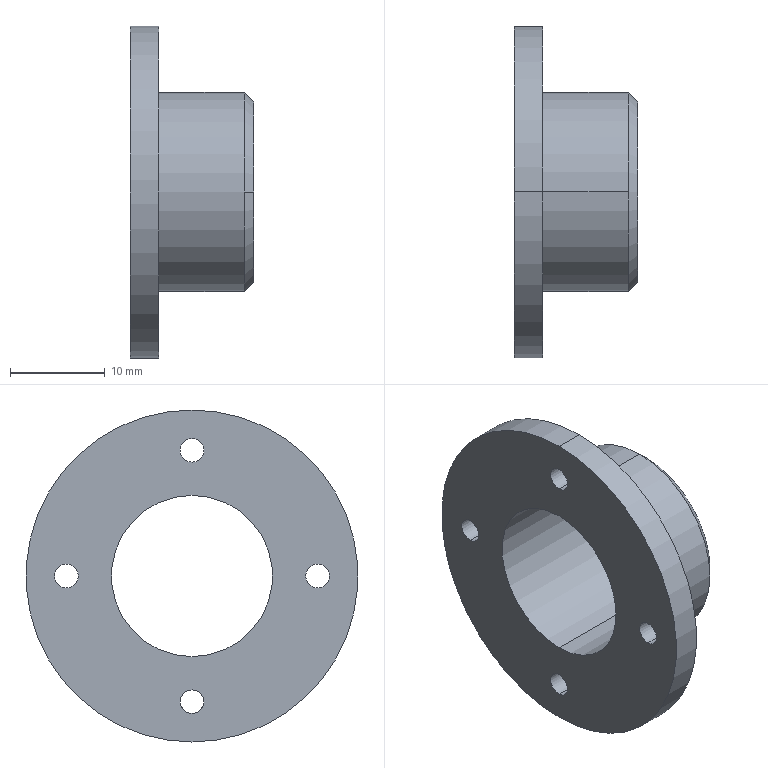Part | SolidWorks | features BaseBody 1 | 1 solid | 27 faces | box 13 x 35 x 35 mm | volume 3307 mm3 | cylinder 14 | cone 10 | plane 3 | commonest cylinder face diameters 2.5 x8 17 x2 21 x2 35 x2
STEP:
#1=CARTESIAN_POINT('',(13.,0.,-8.5));
#2=VERTEX_POINT('',#1);
#3=CARTESIAN_POINT('',(13.,0.,8.5));
#4=VERTEX_POINT('',#3);
#5=CARTESIAN_POINT('',(13.,0.,0.));
#6=DIRECTION('',(-1.,0.,0.));
#7=DIRECTION('',(0.,0.,1.));
#8=AXIS2_PLACEMENT_3D('',#5,#6,#7);
#9=CIRCLE('',#8,8.5);
#10=EDGE_CURVE('',#2,#4,#9,.T.);
#11=ORIENTED_EDGE('',*,*,#10,.F.);
#12=CARTESIAN_POINT('',(0.,0.,-8.5));
#13=VERTEX_POINT('',#12);
#14=CARTESIAN_POINT('',(3.,0.,-8.5));
#15=DIRECTION('',(-1.,0.,0.));
#16=VECTOR('',#15,1000.);
#17=LINE('',#14,#16);
#18=EDGE_CURVE('',#2,#13,#17,.T.);
#19=ORIENTED_EDGE('',*,*,#18,.T.);
#20=CARTESIAN_POINT('',(0.,0.,8.5));
#21=VERTEX_POINT('',#20);
#22=CARTESIAN_POINT('',(0.,0.,0.));
#23=DIRECTION('',(-1.,0.,0.));
#24=DIRECTION('',(0.,0.,1.));
#25=AXIS2_PLACEMENT_3D('',#22,#23,#24);
#26=CIRCLE('',#25,8.5);
#27=EDGE_CURVE('',#13,#21,#26,.T.);
#28=ORIENTED_EDGE('',*,*,#27,.T.);
#29=CARTESIAN_POINT('',(3.,0.,8.5));
#30=DIRECTION('',(-1.,0.,0.));
#31=VECTOR('',#30,1000.);
#32=LINE('',#29,#31);
#33=EDGE_CURVE('',#4,#21,#32,.T.);
#34=ORIENTED_EDGE('',*,*,#33,.F.);
#35=EDGE_LOOP('',(#11,#19,#28,#34));
#36=FACE_OUTER_BOUND('',#35,.T.);
#37=CARTESIAN_POINT('',(3.,0.,0.));
#38=DIRECTION('',(-1.,0.,0.));
#39=DIRECTION('',(0.,0.,1.));
#40=AXIS2_PLACEMENT_3D('',#37,#38,#39);
#41=CYLINDRICAL_SURFACE('',#40,8.5);
#42=ADVANCED_FACE('',(#36),#41,.F.);
#43=CARTESIAN_POINT('',(3.,0.,17.5));
#44=VERTEX_POINT('',#43);
#45=CARTESIAN_POINT('',(3.,0.,-17.5));
#46=VERTEX_POINT('',#45);
#47=CARTESIAN_POINT('',(3.,0.,0.));
#48=DIRECTION('',(-1.,0.,0.));
#49=DIRECTION('',(0.,0.,1.));
#50=AXIS2_PLACEMENT_3D('',#47,#48,#49);
#51=CIRCLE('',#50,17.5);
#52=EDGE_CURVE('',#44,#46,#51,.T.);
#53=ORIENTED_EDGE('',*,*,#52,.T.);
#54=CARTESIAN_POINT('',(0.,0.,-17.5));
#55=VERTEX_POINT('',#54);
#56=CARTESIAN_POINT('',(3.,0.,-17.5));
#57=DIRECTION('',(-1.,0.,0.));
#58=VECTOR('',#57,1000.);
#59=LINE('',#56,#58);
#60=EDGE_CURVE('',#46,#55,#59,.T.);
#61=ORIENTED_EDGE('',*,*,#60,.T.);
#62=CARTESIAN_POINT('',(0.,0.,17.5));
#63=VERTEX_POINT('',#62);
#64=CARTESIAN_POINT('',(0.,0.,0.));
#65=DIRECTION('',(1.,0.,0.));
#66=DIRECTION('',(0.,0.,1.));
#67=AXIS2_PLACEMENT_3D('',#64,#65,#66);
#68=CIRCLE('',#67,17.5);
#69=EDGE_CURVE('',#55,#63,#68,.T.);
#70=ORIENTED_EDGE('',*,*,#69,.T.);
#71=CARTESIAN_POINT('',(3.,0.,17.5));
#72=DIRECTION('',(-1.,0.,0.));
#73=VECTOR('',#72,1000.);
#74=LINE('',#71,#73);
#75=EDGE_CURVE('',#44,#63,#74,.T.);
#76=ORIENTED_EDGE('',*,*,#75,.F.);
#77=EDGE_LOOP('',(#53,#61,#70,#76));
#78=FACE_OUTER_BOUND('',#77,.T.);
#79=CARTESIAN_POINT('',(3.,0.,0.));
#80=DIRECTION('',(-1.,0.,0.));
#81=DIRECTION('',(0.,0.,1.));
#82=AXIS2_PLACEMENT_3D('',#79,#80,#81);
#83=CYLINDRICAL_SURFACE('',#82,17.5);
#84=ADVANCED_FACE('',(#78),#83,.T.);
#85=CARTESIAN_POINT('',(0.,-13.25,-1.25));
#86=VERTEX_POINT('',#85);
#87=CARTESIAN_POINT('',(0.,-13.25,1.25));
#88=VERTEX_POINT('',#87);
#89=CARTESIAN_POINT('',(0.,-13.25,0.));
#90=DIRECTION('',(-1.,0.,0.));
#91=DIRECTION('',(0.,0.,-1.));
#92=AXIS2_PLACEMENT_3D('',#89,#90,#91);
#93=CIRCLE('',#92,1.25);
#94=EDGE_CURVE('',#86,#88,#93,.T.);
#95=ORIENTED_EDGE('',*,*,#94,.T.);
#96=CARTESIAN_POINT('',(2.725,-13.25,1.25));
#97=VERTEX_POINT('',#96);
#98=CARTESIAN_POINT('',(3.,-13.25,1.25));
#99=DIRECTION('',(1.,0.,0.));
#100=VECTOR('',#99,1000.);
#101=LINE('',#98,#100);
#102=EDGE_CURVE('',#88,#97,#101,.T.);
#103=ORIENTED_EDGE('',*,*,#102,.T.);
#104=CARTESIAN_POINT('',(2.725,-13.25,-1.25));
#105=VERTEX_POINT('',#104);
#106=CARTESIAN_POINT('',(2.725,-13.25,0.));
#107=DIRECTION('',(-1.,0.,0.));
#108=DIRECTION('',(0.,0.,-1.));
#109=AXIS2_PLACEMENT_3D('',#106,#107,#108);
#110=CIRCLE('',#109,1.25);
#111=EDGE_CURVE('',#105,#97,#110,.T.);
#112=ORIENTED_EDGE('',*,*,#111,.F.);
#113=CARTESIAN_POINT('',(3.,-13.25,-1.25));
#114=DIRECTION('',(1.,0.,0.));
#115=VECTOR('',#114,1000.);
#116=LINE('',#113,#115);
#117=EDGE_CURVE('',#86,#105,#116,.T.);
#118=ORIENTED_EDGE('',*,*,#117,.F.);
#119=EDGE_LOOP('',(#95,#103,#112,#118));
#120=FACE_OUTER_BOUND('',#119,.T.);
#121=CARTESIAN_POINT('',(3.,-13.25,0.));
#122=DIRECTION('',(1.,0.,0.));
#123=DIRECTION('',(0.,0.,-1.));
#124=AXIS2_PLACEMENT_3D('',#121,#122,#123);
#125=CYLINDRICAL_SURFACE('',#124,1.25);
#126=ADVANCED_FACE('',(#120),#125,.F.);
#127=CARTESIAN_POINT('',(0.,0.,12.));
#128=VERTEX_POINT('',#127);
#129=CARTESIAN_POINT('',(0.,0.,14.5));
#130=VERTEX_POINT('',#129);
#131=CARTESIAN_POINT('',(0.,0.,13.25));
#132=DIRECTION('',(-1.,0.,0.));
#133=DIRECTION('',(0.,0.,-1.));
#134=AXIS2_PLACEMENT_3D('',#131,#132,#133);
#135=CIRCLE('',#134,1.25);
#136=EDGE_CURVE('',#128,#130,#135,.T.);
#137=ORIENTED_EDGE('',*,*,#136,.T.);
#138=CARTESIAN_POINT('',(2.725,0.,14.5));
#139=VERTEX_POINT('',#138);
#140=CARTESIAN_POINT('',(3.,0.,14.5));
#141=DIRECTION('',(1.,0.,0.));
#142=VECTOR('',#141,1000.);
#143=LINE('',#140,#142);
#144=EDGE_CURVE('',#130,#139,#143,.T.);
#145=ORIENTED_EDGE('',*,*,#144,.T.);
#146=CARTESIAN_POINT('',(2.725,0.,12.));
#147=VERTEX_POINT('',#146);
#148=CARTESIAN_POINT('',(2.725,0.,13.25));
#149=DIRECTION('',(-1.,0.,0.));
#150=DIRECTION('',(0.,0.,-1.));
#151=AXIS2_PLACEMENT_3D('',#148,#149,#150);
#152=CIRCLE('',#151,1.25);
#153=EDGE_CURVE('',#147,#139,#152,.T.);
#154=ORIENTED_EDGE('',*,*,#153,.F.);
#155=CARTESIAN_POINT('',(3.,0.,12.));
#156=DIRECTION('',(1.,0.,0.));
#157=VECTOR('',#156,1000.);
#158=LINE('',#155,#157);
#159=EDGE_CURVE('',#128,#147,#158,.T.);
#160=ORIENTED_EDGE('',*,*,#159,.F.);
#161=EDGE_LOOP('',(#137,#145,#154,#160));
#162=FACE_OUTER_BOUND('',#161,.T.);
#163=CARTESIAN_POINT('',(3.,0.,13.25));
#164=DIRECTION('',(1.,0.,0.));
#165=DIRECTION('',(0.,0.,-1.));
#166=AXIS2_PLACEMENT_3D('',#163,#164,#165);
#167=CYLINDRICAL_SURFACE('',#166,1.25);
#168=ADVANCED_FACE('',(#162),#167,.F.);
#169=CARTESIAN_POINT('',(0.,0.,-14.5));
#170=VERTEX_POINT('',#169);
#171=CARTESIAN_POINT('',(0.,0.,-12.));
#172=VERTEX_POINT('',#171);
#173=CARTESIAN_POINT('',(0.,0.,-13.25));
#174=DIRECTION('',(-1.,0.,0.));
#175=DIRECTION('',(0.,0.,-1.));
#176=AXIS2_PLACEMENT_3D('',#173,#174,#175);
#177=CIRCLE('',#176,1.25);
#178=EDGE_CURVE('',#170,#172,#177,.T.);
#179=ORIENTED_EDGE('',*,*,#178,.T.);
#180=CARTESIAN_POINT('',(2.725,0.,-12.));
#181=VERTEX_POINT('',#180);
#182=CARTESIAN_POINT('',(3.,0.,-12.));
#183=DIRECTION('',(1.,0.,0.));
#184=VECTOR('',#183,1000.);
#185=LINE('',#182,#184);
#186=EDGE_CURVE('',#172,#181,#185,.T.);
#187=ORIENTED_EDGE('',*,*,#186,.T.);
#188=CARTESIAN_POINT('',(2.725,-1.25,-13.25));
#189=VERTEX_POINT('',#188);
#190=CARTESIAN_POINT('',(2.725,0.,-13.25));
#191=DIRECTION('',(-1.,0.,0.));
#192=DIRECTION('',(0.,0.,-1.));
#193=AXIS2_PLACEMENT_3D('',#190,#191,#192);
#194=CIRCLE('',#193,1.25);
#195=EDGE_CURVE('',#189,#181,#194,.T.);
#196=ORIENTED_EDGE('',*,*,#195,.F.);
#197=CARTESIAN_POINT('',(2.725,0.,-14.5));
#198=VERTEX_POINT('',#197);
#199=CARTESIAN_POINT('',(2.725,0.,-13.25));
#200=DIRECTION('',(-1.,0.,0.));
#201=DIRECTION('',(0.,0.,-1.));
#202=AXIS2_PLACEMENT_3D('',#199,#200,#201);
#203=CIRCLE('',#202,1.25);
#204=EDGE_CURVE('',#198,#189,#203,.T.);
#205=ORIENTED_EDGE('',*,*,#204,.F.);
#206=CARTESIAN_POINT('',(3.,0.,-14.5));
#207=DIRECTION('',(1.,0.,0.));
#208=VECTOR('',#207,1000.);
#209=LINE('',#206,#208);
#210=EDGE_CURVE('',#170,#198,#209,.T.);
#211=ORIENTED_EDGE('',*,*,#210,.F.);
#212=EDGE_LOOP('',(#179,#187,#196,#205,#211));
#213=FACE_OUTER_BOUND('',#212,.T.);
#214=CARTESIAN_POINT('',(3.,0.,-13.25));
#215=DIRECTION('',(1.,0.,0.));
#216=DIRECTION('',(0.,0.,-1.));
#217=AXIS2_PLACEMENT_3D('',#214,#215,#216);
#218=CYLINDRICAL_SURFACE('',#217,1.25);
#219=ADVANCED_FACE('',(#213),#218,.F.);
#220=CARTESIAN_POINT('',(0.,13.25,-1.25));
#221=VERTEX_POINT('',#220);
#222=CARTESIAN_POINT('',(0.,13.25,1.25));
#223=VERTEX_POINT('',#222);
#224=CARTESIAN_POINT('',(0.,13.25,0.));
#225=DIRECTION('',(-1.,0.,0.));
#226=DIRECTION('',(0.,0.,-1.));
#227=AXIS2_PLACEMENT_3D('',#224,#225,#226);
#228=CIRCLE('',#227,1.25);
#229=EDGE_CURVE('',#221,#223,#228,.T.);
#230=ORIENTED_EDGE('',*,*,#229,.T.);
#231=CARTESIAN_POINT('',(2.725,13.25,1.25));
#232=VERTEX_POINT('',#231);
#233=CARTESIAN_POINT('',(3.,13.25,1.25));
#234=DIRECTION('',(1.,0.,0.));
#235=VECTOR('',#234,1000.);
#236=LINE('',#233,#235);
#237=EDGE_CURVE('',#223,#232,#236,.T.);
#238=ORIENTED_EDGE('',*,*,#237,.T.);
#239=CARTESIAN_POINT('',(2.725,13.25,-1.25));
#240=VERTEX_POINT('',#239);
#241=CARTESIAN_POINT('',(2.725,13.25,0.));
#242=DIRECTION('',(-1.,0.,0.));
#243=DIRECTION('',(0.,0.,-1.));
#244=AXIS2_PLACEMENT_3D('',#241,#242,#243);
#245=CIRCLE('',#244,1.25);
#246=EDGE_CURVE('',#240,#232,#245,.T.);
#247=ORIENTED_EDGE('',*,*,#246,.F.);
#248=CARTESIAN_POINT('',(3.,13.25,-1.25));
#249=DIRECTION('',(1.,0.,0.));
#250=VECTOR('',#249,1000.);
#251=LINE('',#248,#250);
#252=EDGE_CURVE('',#221,#240,#251,.T.);
#253=ORIENTED_EDGE('',*,*,#252,.F.);
#254=EDGE_LOOP('',(#230,#238,#247,#253));
#255=FACE_OUTER_BOUND('',#254,.T.);
#256=CARTESIAN_POINT('',(3.,13.25,0.));
#257=DIRECTION('',(1.,0.,0.));
#258=DIRECTION('',(0.,0.,-1.));
#259=AXIS2_PLACEMENT_3D('',#256,#257,#258);
#260=CYLINDRICAL_SURFACE('',#259,1.25);
#261=ADVANCED_FACE('',(#255),#260,.F.);
#262=ORIENTED_EDGE('',*,*,#111,.T.);
#263=CARTESIAN_POINT('',(3.,-13.25,1.525));
#264=VERTEX_POINT('',#263);
#265=CARTESIAN_POINT('',(3.,-13.25,1.525));
#266=DIRECTION('',(0.7071,0.,0.7071));
#267=VECTOR('',#266,1000.);
#268=LINE('',#265,#267);
#269=EDGE_CURVE('',#97,#264,#268,.T.);
#270=ORIENTED_EDGE('',*,*,#269,.T.);
#271=CARTESIAN_POINT('',(3.,-13.25,-1.525));
#272=VERTEX_POINT('',#271);
#273=CARTESIAN_POINT('',(3.,-13.25,0.));
#274=DIRECTION('',(-1.,0.,0.));
#275=DIRECTION('',(0.,0.,-1.));
#276=AXIS2_PLACEMENT_3D('',#273,#274,#275);
#277=CIRCLE('',#276,1.525);
#278=EDGE_CURVE('',#272,#264,#277,.T.);
#279=ORIENTED_EDGE('',*,*,#278,.F.);
#280=CARTESIAN_POINT('',(3.,-13.25,-1.525));
#281=DIRECTION('',(0.7071,0.,-0.7071));
#282=VECTOR('',#281,1000.);
#283=LINE('',#280,#282);
#284=EDGE_CURVE('',#105,#272,#283,.T.);
#285=ORIENTED_EDGE('',*,*,#284,.F.);
#286=EDGE_LOOP('',(#262,#270,#279,#285));
#287=FACE_OUTER_BOUND('',#286,.T.);
#288=CARTESIAN_POINT('',(3.,-13.25,0.));
#289=DIRECTION('',(1.,0.,0.));
#290=DIRECTION('',(0.,0.,-1.));
#291=AXIS2_PLACEMENT_3D('',#288,#289,#290);
#292=CONICAL_SURFACE('',#291,1.525,0.7854);
#293=ADVANCED_FACE('',(#287),#292,.F.);
#294=ORIENTED_EDGE('',*,*,#153,.T.);
#295=CARTESIAN_POINT('',(3.,0.,14.775));
#296=VERTEX_POINT('',#295);
#297=CARTESIAN_POINT('',(3.,0.,14.775));
#298=DIRECTION('',(0.7071,0.,0.7071));
#299=VECTOR('',#298,1000.);
#300=LINE('',#297,#299);
#301=EDGE_CURVE('',#139,#296,#300,.T.);
#302=ORIENTED_EDGE('',*,*,#301,.T.);
#303=CARTESIAN_POINT('',(3.,0.,11.725));
#304=VERTEX_POINT('',#303);
#305=CARTESIAN_POINT('',(3.,0.,13.25));
#306=DIRECTION('',(-1.,0.,0.));
#307=DIRECTION('',(0.,0.,-1.));
#308=AXIS2_PLACEMENT_3D('',#305,#306,#307);
#309=CIRCLE('',#308,1.525);
#310=EDGE_CURVE('',#304,#296,#309,.T.);
#311=ORIENTED_EDGE('',*,*,#310,.F.);
#312=CARTESIAN_POINT('',(3.,0.,11.725));
#313=DIRECTION('',(0.7071,0.,-0.7071));
#314=VECTOR('',#313,1000.);
#315=LINE('',#312,#314);
#316=EDGE_CURVE('',#147,#304,#315,.T.);
#317=ORIENTED_EDGE('',*,*,#316,.F.);
#318=EDGE_LOOP('',(#294,#302,#311,#317));
#319=FACE_OUTER_BOUND('',#318,.T.);
#320=CARTESIAN_POINT('',(3.,0.,13.25));
#321=DIRECTION('',(1.,0.,0.));
#322=DIRECTION('',(0.,0.,-1.));
#323=AXIS2_PLACEMENT_3D('',#320,#321,#322);
#324=CONICAL_SURFACE('',#323,1.525,0.7854);
#325=ADVANCED_FACE('',(#319),#324,.F.);
#326=CARTESIAN_POINT('',(2.725,1.25,-13.25));
#327=VERTEX_POINT('',#326);
#328=CARTESIAN_POINT('',(2.725,0.,-13.25));
#329=DIRECTION('',(-1.,0.,0.));
#330=DIRECTION('',(0.,0.,-1.));
#331=AXIS2_PLACEMENT_3D('',#328,#329,#330);
#332=CIRCLE('',#331,1.25);
#333=EDGE_CURVE('',#327,#198,#332,.T.);
#334=ORIENTED_EDGE('',*,*,#333,.T.);
#335=ORIENTED_EDGE('',*,*,#204,.T.);
#336=CARTESIAN_POINT('',(3.,-1.525,-13.25));
#337=VERTEX_POINT('',#336);
#338=CARTESIAN_POINT('',(3.,-1.525,-13.25));
#339=DIRECTION('',(0.7071,-0.7071,0.));
#340=VECTOR('',#339,1000.);
#341=LINE('',#338,#340);
#342=EDGE_CURVE('',#189,#337,#341,.T.);
#343=ORIENTED_EDGE('',*,*,#342,.T.);
#344=CARTESIAN_POINT('',(3.,1.525,-13.25));
#345=VERTEX_POINT('',#344);
#346=CARTESIAN_POINT('',(3.,0.,-13.25));
#347=DIRECTION('',(-1.,0.,0.));
#348=DIRECTION('',(0.,1.,0.));
#349=AXIS2_PLACEMENT_3D('',#346,#347,#348);
#350=CIRCLE('',#349,1.525);
#351=EDGE_CURVE('',#345,#337,#350,.T.);
#352=ORIENTED_EDGE('',*,*,#351,.F.);
#353=CARTESIAN_POINT('',(3.,1.525,-13.25));
#354=DIRECTION('',(0.7071,0.7071,0.));
#355=VECTOR('',#354,1000.);
#356=LINE('',#353,#355);
#357=EDGE_CURVE('',#327,#345,#356,.T.);
#358=ORIENTED_EDGE('',*,*,#357,.F.);
#359=EDGE_LOOP('',(#334,#335,#343,#352,#358));
#360=FACE_OUTER_BOUND('',#359,.T.);
#361=CARTESIAN_POINT('',(3.,0.,-13.25));
#362=DIRECTION('',(1.,0.,0.));
#363=DIRECTION('',(0.,1.,0.));
#364=AXIS2_PLACEMENT_3D('',#361,#362,#363);
#365=CONICAL_SURFACE('',#364,1.525,0.7854);
#366=ADVANCED_FACE('',(#360),#365,.F.);
#367=ORIENTED_EDGE('',*,*,#246,.T.);
#368=CARTESIAN_POINT('',(3.,13.25,1.525));
#369=VERTEX_POINT('',#368);
#370=CARTESIAN_POINT('',(3.,13.25,1.525));
#371=DIRECTION('',(0.7071,0.,0.7071));
#372=VECTOR('',#371,1000.);
#373=LINE('',#370,#372);
#374=EDGE_CURVE('',#232,#369,#373,.T.);
#375=ORIENTED_EDGE('',*,*,#374,.T.);
#376=CARTESIAN_POINT('',(3.,13.25,-1.525));
#377=VERTEX_POINT('',#376);
#378=CARTESIAN_POINT('',(3.,13.25,0.));
#379=DIRECTION('',(-1.,0.,0.));
#380=DIRECTION('',(0.,0.,-1.));
#381=AXIS2_PLACEMENT_3D('',#378,#379,#380);
#382=CIRCLE('',#381,1.525);
#383=EDGE_CURVE('',#377,#369,#382,.T.);
#384=ORIENTED_EDGE('',*,*,#383,.F.);
#385=CARTESIAN_POINT('',(3.,13.25,-1.525));
#386=DIRECTION('',(0.7071,0.,-0.7071));
#387=VECTOR('',#386,1000.);
#388=LINE('',#385,#387);
#389=EDGE_CURVE('',#240,#377,#388,.T.);
#390=ORIENTED_EDGE('',*,*,#389,.F.);
#391=EDGE_LOOP('',(#367,#375,#384,#390));
#392=FACE_OUTER_BOUND('',#391,.T.);
#393=CARTESIAN_POINT('',(3.,13.25,0.));
#394=DIRECTION('',(1.,0.,0.));
#395=DIRECTION('',(0.,0.,-1.));
#396=AXIS2_PLACEMENT_3D('',#393,#394,#395);
#397=CONICAL_SURFACE('',#396,1.525,0.7854);
#398=ADVANCED_FACE('',(#392),#397,.F.);
#399=CARTESIAN_POINT('',(13.,9.5,0.));
#400=VERTEX_POINT('',#399);
#401=CARTESIAN_POINT('',(13.,-9.5,0.));
#402=VERTEX_POINT('',#401);
#403=CARTESIAN_POINT('',(13.,0.,0.));
#404=DIRECTION('',(1.,0.,0.));
#405=DIRECTION('',(0.,-1.,0.));
#406=AXIS2_PLACEMENT_3D('',#403,#404,#405);
#407=CIRCLE('',#406,9.5);
#408=EDGE_CURVE('',#400,#402,#407,.T.);
#409=ORIENTED_EDGE('',*,*,#408,.F.);
#410=CARTESIAN_POINT('',(12.,10.5,0.));
#411=VERTEX_POINT('',#410);
#412=CARTESIAN_POINT('',(12.,10.5,0.));
#413=DIRECTION('',(-0.7071,0.7071,0.));
#414=VECTOR('',#413,1000.);
#415=LINE('',#412,#414);
#416=EDGE_CURVE('',#400,#411,#415,.T.);
#417=ORIENTED_EDGE('',*,*,#416,.T.);
#418=CARTESIAN_POINT('',(12.,0.,10.5));
#419=VERTEX_POINT('',#418);
#420=CARTESIAN_POINT('',(12.,0.,0.));
#421=DIRECTION('',(1.,0.,0.));
#422=DIRECTION('',(0.,0.,1.));
#423=AXIS2_PLACEMENT_3D('',#420,#421,#422);
#424=CIRCLE('',#423,10.5);
#425=EDGE_CURVE('',#411,#419,#424,.T.);
#426=ORIENTED_EDGE('',*,*,#425,.T.);
#427=CARTESIAN_POINT('',(12.,-10.5,0.));
#428=VERTEX_POINT('',#427);
#429=CARTESIAN_POINT('',(12.,0.,0.));
#430=DIRECTION('',(1.,0.,0.));
#431=DIRECTION('',(0.,0.,1.));
#432=AXIS2_PLACEMENT_3D('',#429,#430,#431);
#433=CIRCLE('',#432,10.5);
#434=EDGE_CURVE('',#419,#428,#433,.T.);
#435=ORIENTED_EDGE('',*,*,#434,.T.);
#436=CARTESIAN_POINT('',(12.,-10.5,0.));
#437=DIRECTION('',(-0.7071,-0.7071,0.));
#438=VECTOR('',#437,1000.);
#439=LINE('',#436,#438);
#440=EDGE_CURVE('',#402,#428,#439,.T.);
#441=ORIENTED_EDGE('',*,*,#440,.F.);
#442=EDGE_LOOP('',(#409,#417,#426,#435,#441));
#443=FACE_OUTER_BOUND('',#442,.T.);
#444=CARTESIAN_POINT('',(12.,0.,0.));
#445=DIRECTION('',(-1.,0.,0.));
#446=DIRECTION('',(0.,-1.,0.));
#447=AXIS2_PLACEMENT_3D('',#444,#445,#446);
#448=CONICAL_SURFACE('',#447,10.5,0.7854);
#449=ADVANCED_FACE('',(#443),#448,.T.);
#450=CARTESIAN_POINT('',(12.,0.,-10.5));
#451=VERTEX_POINT('',#450);
#452=CARTESIAN_POINT('',(12.,0.,0.));
#453=DIRECTION('',(1.,0.,0.));
#454=DIRECTION('',(0.,0.,1.));
#455=AXIS2_PLACEMENT_3D('',#452,#453,#454);
#456=CIRCLE('',#455,10.5);
#457=EDGE_CURVE('',#451,#411,#456,.T.);
#458=ORIENTED_EDGE('',*,*,#457,.F.);
#459=CARTESIAN_POINT('',(3.,0.,-10.5));
#460=VERTEX_POINT('',#459);
#461=CARTESIAN_POINT('',(13.,0.,-10.5));
#462=DIRECTION('',(-1.,0.,0.));
#463=VECTOR('',#462,1000.);
#464=LINE('',#461,#463);
#465=EDGE_CURVE('',#451,#460,#464,.T.);
#466=ORIENTED_EDGE('',*,*,#465,.T.);
#467=CARTESIAN_POINT('',(3.,0.,10.5));
#468=VERTEX_POINT('',#467);
#469=CARTESIAN_POINT('',(3.,0.,0.));
#470=DIRECTION('',(-1.,0.,0.));
#471=DIRECTION('',(0.,0.,1.));
#472=AXIS2_PLACEMENT_3D('',#469,#470,#471);
#473=CIRCLE('',#472,10.5);
#474=EDGE_CURVE('',#468,#460,#473,.T.);
#475=ORIENTED_EDGE('',*,*,#474,.F.);
#476=CARTESIAN_POINT('',(13.,0.,10.5));
#477=DIRECTION('',(-1.,0.,0.));
#478=VECTOR('',#477,1000.);
#479=LINE('',#476,#478);
#480=EDGE_CURVE('',#419,#468,#479,.T.);
#481=ORIENTED_EDGE('',*,*,#480,.F.);
#482=ORIENTED_EDGE('',*,*,#425,.F.);
#483=EDGE_LOOP('',(#458,#466,#475,#481,#482));
#484=FACE_OUTER_BOUND('',#483,.T.);
#485=CARTESIAN_POINT('',(13.,0.,0.));
#486=DIRECTION('',(-1.,0.,0.));
#487=DIRECTION('',(0.,0.,1.));
#488=AXIS2_PLACEMENT_3D('',#485,#486,#487);
#489=CYLINDRICAL_SURFACE('',#488,10.5);
#490=ADVANCED_FACE('',(#484),#489,.T.);
#491=CARTESIAN_POINT('',(0.,0.,0.));
#492=DIRECTION('',(-1.,0.,0.));
#493=DIRECTION('',(0.,0.,1.));
#494=AXIS2_PLACEMENT_3D('',#491,#492,#493);
#495=CIRCLE('',#494,8.5);
#496=EDGE_CURVE('',#21,#13,#495,.T.);
#497=ORIENTED_EDGE('',*,*,#496,.F.);
#498=ORIENTED_EDGE('',*,*,#27,.F.);
#499=EDGE_LOOP('',(#497,#498));
#500=FACE_BOUND('',#499,.T.);
#501=CARTESIAN_POINT('',(0.,0.,0.));
#502=DIRECTION('',(1.,0.,0.));
#503=DIRECTION('',(0.,0.,1.));
#504=AXIS2_PLACEMENT_3D('',#501,#502,#503);
#505=CIRCLE('',#504,17.5);
#506=EDGE_CURVE('',#63,#55,#505,.T.);
#507=ORIENTED_EDGE('',*,*,#506,.F.);
#508=ORIENTED_EDGE('',*,*,#69,.F.);
#509=EDGE_LOOP('',(#507,#508));
#510=FACE_OUTER_BOUND('',#509,.T.);
#511=ORIENTED_EDGE('',*,*,#94,.F.);
#512=CARTESIAN_POINT('',(0.,-13.25,0.));
#513=DIRECTION('',(-1.,0.,0.));
#514=DIRECTION('',(0.,0.,-1.));
#515=AXIS2_PLACEMENT_3D('',#512,#513,#514);
#516=CIRCLE('',#515,1.25);
#517=EDGE_CURVE('',#88,#86,#516,.T.);
#518=ORIENTED_EDGE('',*,*,#517,.F.);
#519=EDGE_LOOP('',(#511,#518));
#520=FACE_BOUND('',#519,.T.);
#521=ORIENTED_EDGE('',*,*,#136,.F.);
#522=CARTESIAN_POINT('',(0.,0.,13.25));
#523=DIRECTION('',(-1.,0.,0.));
#524=DIRECTION('',(0.,0.,-1.));
#525=AXIS2_PLACEMENT_3D('',#522,#523,#524);
#526=CIRCLE('',#525,1.25);
#527=EDGE_CURVE('',#130,#128,#526,.T.);
#528=ORIENTED_EDGE('',*,*,#527,.F.);
#529=EDGE_LOOP('',(#521,#528));
#530=FACE_BOUND('',#529,.T.);
#531=ORIENTED_EDGE('',*,*,#178,.F.);
#532=CARTESIAN_POINT('',(0.,0.,-13.25));
#533=DIRECTION('',(-1.,0.,0.));
#534=DIRECTION('',(0.,0.,-1.));
#535=AXIS2_PLACEMENT_3D('',#532,#533,#534);
#536=CIRCLE('',#535,1.25);
#537=EDGE_CURVE('',#172,#170,#536,.T.);
#538=ORIENTED_EDGE('',*,*,#537,.F.);
#539=EDGE_LOOP('',(#531,#538));
#540=FACE_BOUND('',#539,.T.);
#541=ORIENTED_EDGE('',*,*,#229,.F.);
#542=CARTESIAN_POINT('',(0.,13.25,0.));
#543=DIRECTION('',(-1.,0.,0.));
#544=DIRECTION('',(0.,0.,-1.));
#545=AXIS2_PLACEMENT_3D('',#542,#543,#544);
#546=CIRCLE('',#545,1.25);
#547=EDGE_CURVE('',#223,#221,#546,.T.);
#548=ORIENTED_EDGE('',*,*,#547,.F.);
#549=EDGE_LOOP('',(#541,#548));
#550=FACE_BOUND('',#549,.T.);
#551=CARTESIAN_POINT('',(0.,0.,0.));
#552=DIRECTION('',(1.,0.,0.));
#553=DIRECTION('',(0.,0.,-1.));
#554=AXIS2_PLACEMENT_3D('',#551,#552,#553);
#555=PLANE('',#554);
#556=ADVANCED_FACE('',(#500,#510,#520,#530,#540,#550),#555,.F.);
#557=ORIENTED_EDGE('',*,*,#18,.F.);
#558=CARTESIAN_POINT('',(13.,0.,0.));
#559=DIRECTION('',(-1.,0.,0.));
#560=DIRECTION('',(0.,0.,1.));
#561=AXIS2_PLACEMENT_3D('',#558,#559,#560);
#562=CIRCLE('',#561,8.5);
#563=EDGE_CURVE('',#4,#2,#562,.T.);
#564=ORIENTED_EDGE('',*,*,#563,.F.);
#565=ORIENTED_EDGE('',*,*,#33,.T.);
#566=ORIENTED_EDGE('',*,*,#496,.T.);
#567=EDGE_LOOP('',(#557,#564,#565,#566));
#568=FACE_OUTER_BOUND('',#567,.T.);
#569=CARTESIAN_POINT('',(3.,0.,0.));
#570=DIRECTION('',(-1.,0.,0.));
#571=DIRECTION('',(0.,0.,1.));
#572=AXIS2_PLACEMENT_3D('',#569,#570,#571);
#573=CYLINDRICAL_SURFACE('',#572,8.5);
#574=ADVANCED_FACE('',(#568),#573,.F.);
#575=ORIENTED_EDGE('',*,*,#60,.F.);
#576=CARTESIAN_POINT('',(3.,0.,0.));
#577=DIRECTION('',(-1.,0.,0.));
#578=DIRECTION('',(0.,0.,1.));
#579=AXIS2_PLACEMENT_3D('',#576,#577,#578);
#580=CIRCLE('',#579,17.5);
#581=EDGE_CURVE('',#46,#44,#580,.T.);
#582=ORIENTED_EDGE('',*,*,#581,.T.);
#583=ORIENTED_EDGE('',*,*,#75,.T.);
#584=ORIENTED_EDGE('',*,*,#506,.T.);
#585=EDGE_LOOP('',(#575,#582,#583,#584));
#586=FACE_OUTER_BOUND('',#585,.T.);
#587=CARTESIAN_POINT('',(3.,0.,0.));
#588=DIRECTION('',(-1.,0.,0.));
#589=DIRECTION('',(0.,0.,1.));
#590=AXIS2_PLACEMENT_3D('',#587,#588,#589);
#591=CYLINDRICAL_SURFACE('',#590,17.5);
#592=ADVANCED_FACE('',(#586),#591,.T.);
#593=ORIENTED_EDGE('',*,*,#102,.F.);
#594=ORIENTED_EDGE('',*,*,#517,.T.);
#595=ORIENTED_EDGE('',*,*,#117,.T.);
#596=CARTESIAN_POINT('',(2.725,-13.25,0.));
#597=DIRECTION('',(-1.,0.,0.));
#598=DIRECTION('',(0.,0.,-1.));
#599=AXIS2_PLACEMENT_3D('',#596,#597,#598);
#600=CIRCLE('',#599,1.25);
#601=EDGE_CURVE('',#97,#105,#600,.T.);
#602=ORIENTED_EDGE('',*,*,#601,.F.);
#603=EDGE_LOOP('',(#593,#594,#595,#602));
#604=FACE_OUTER_BOUND('',#603,.T.);
#605=CARTESIAN_POINT('',(3.,-13.25,0.));
#606=DIRECTION('',(1.,0.,0.));
#607=DIRECTION('',(0.,0.,-1.));
#608=AXIS2_PLACEMENT_3D('',#605,#606,#607);
#609=CYLINDRICAL_SURFACE('',#608,1.25);
#610=ADVANCED_FACE('',(#604),#609,.F.);
#611=ORIENTED_EDGE('',*,*,#144,.F.);
#612=ORIENTED_EDGE('',*,*,#527,.T.);
#613=ORIENTED_EDGE('',*,*,#159,.T.);
#614=CARTESIAN_POINT('',(2.725,0.,13.25));
#615=DIRECTION('',(-1.,0.,0.));
#616=DIRECTION('',(0.,0.,-1.));
#617=AXIS2_PLACEMENT_3D('',#614,#615,#616);
#618=CIRCLE('',#617,1.25);
#619=EDGE_CURVE('',#139,#147,#618,.T.);
#620=ORIENTED_EDGE('',*,*,#619,.F.);
#621=EDGE_LOOP('',(#611,#612,#613,#620));
#622=FACE_OUTER_BOUND('',#621,.T.);
#623=CARTESIAN_POINT('',(3.,0.,13.25));
#624=DIRECTION('',(1.,0.,0.));
#625=DIRECTION('',(0.,0.,-1.));
#626=AXIS2_PLACEMENT_3D('',#623,#624,#625);
#627=CYLINDRICAL_SURFACE('',#626,1.25);
#628=ADVANCED_FACE('',(#622),#627,.F.);
#629=ORIENTED_EDGE('',*,*,#186,.F.);
#630=ORIENTED_EDGE('',*,*,#537,.T.);
#631=ORIENTED_EDGE('',*,*,#210,.T.);
#632=ORIENTED_EDGE('',*,*,#333,.F.);
#633=CARTESIAN_POINT('',(2.725,0.,-13.25));
#634=DIRECTION('',(-1.,0.,0.));
#635=DIRECTION('',(0.,0.,-1.));
#636=AXIS2_PLACEMENT_3D('',#633,#634,#635);
#637=CIRCLE('',#636,1.25);
#638=EDGE_CURVE('',#181,#327,#637,.T.);
#639=ORIENTED_EDGE('',*,*,#638,.F.);
#640=EDGE_LOOP('',(#629,#630,#631,#632,#639));
#641=FACE_OUTER_BOUND('',#640,.T.);
#642=CARTESIAN_POINT('',(3.,0.,-13.25));
#643=DIRECTION('',(1.,0.,0.));
#644=DIRECTION('',(0.,0.,-1.));
#645=AXIS2_PLACEMENT_3D('',#642,#643,#644);
#646=CYLINDRICAL_SURFACE('',#645,1.25);
#647=ADVANCED_FACE('',(#641),#646,.F.);
#648=ORIENTED_EDGE('',*,*,#237,.F.);
#649=ORIENTED_EDGE('',*,*,#547,.T.);
#650=ORIENTED_EDGE('',*,*,#252,.T.);
#651=CARTESIAN_POINT('',(2.725,13.25,0.));
#652=DIRECTION('',(-1.,0.,0.));
#653=DIRECTION('',(0.,0.,-1.));
#654=AXIS2_PLACEMENT_3D('',#651,#652,#653);
#655=CIRCLE('',#654,1.25);
#656=EDGE_CURVE('',#232,#240,#655,.T.);
#657=ORIENTED_EDGE('',*,*,#656,.F.);
#658=EDGE_LOOP('',(#648,#649,#650,#657));
#659=FACE_OUTER_BOUND('',#658,.T.);
#660=CARTESIAN_POINT('',(3.,13.25,0.));
#661=DIRECTION('',(1.,0.,0.));
#662=DIRECTION('',(0.,0.,-1.));
#663=AXIS2_PLACEMENT_3D('',#660,#661,#662);
#664=CYLINDRICAL_SURFACE('',#663,1.25);
#665=ADVANCED_FACE('',(#659),#664,.F.);
#666=ORIENTED_EDGE('',*,*,#563,.T.);
#667=ORIENTED_EDGE('',*,*,#10,.T.);
#668=EDGE_LOOP('',(#666,#667));
#669=FACE_BOUND('',#668,.T.);
#670=CARTESIAN_POINT('',(13.,0.,0.));
#671=DIRECTION('',(1.,0.,0.));
#672=DIRECTION('',(0.,-1.,0.));
#673=AXIS2_PLACEMENT_3D('',#670,#671,#672);
#674=CIRCLE('',#673,9.5);
#675=EDGE_CURVE('',#402,#400,#674,.T.);
#676=ORIENTED_EDGE('',*,*,#675,.T.);
#677=ORIENTED_EDGE('',*,*,#408,.T.);
#678=EDGE_LOOP('',(#676,#677));
#679=FACE_OUTER_BOUND('',#678,.T.);
#680=CARTESIAN_POINT('',(13.,0.,0.));
#681=DIRECTION('',(1.,0.,0.));
#682=DIRECTION('',(0.,0.,-1.));
#683=AXIS2_PLACEMENT_3D('',#680,#681,#682);
#684=PLANE('',#683);
#685=ADVANCED_FACE('',(#669,#679),#684,.T.);
#686=ORIENTED_EDGE('',*,*,#474,.T.);
#687=CARTESIAN_POINT('',(3.,0.,0.));
#688=DIRECTION('',(-1.,0.,0.));
#689=DIRECTION('',(0.,0.,1.));
#690=AXIS2_PLACEMENT_3D('',#687,#688,#689);
#691=CIRCLE('',#690,10.5);
#692=EDGE_CURVE('',#460,#468,#691,.T.);
#693=ORIENTED_EDGE('',*,*,#692,.T.);
#694=EDGE_LOOP('',(#686,#693));
#695=FACE_BOUND('',#694,.T.);
#696=ORIENTED_EDGE('',*,*,#52,.F.);
#697=ORIENTED_EDGE('',*,*,#581,.F.);
#698=EDGE_LOOP('',(#696,#697));
#699=FACE_OUTER_BOUND('',#698,.T.);
#700=ORIENTED_EDGE('',*,*,#278,.T.);
#701=CARTESIAN_POINT('',(3.,-13.25,0.));
#702=DIRECTION('',(-1.,0.,0.));
#703=DIRECTION('',(0.,0.,-1.));
#704=AXIS2_PLACEMENT_3D('',#701,#702,#703);
#705=CIRCLE('',#704,1.525);
#706=EDGE_CURVE('',#264,#272,#705,.T.);
#707=ORIENTED_EDGE('',*,*,#706,.T.);
#708=EDGE_LOOP('',(#700,#707));
#709=FACE_BOUND('',#708,.T.);
#710=ORIENTED_EDGE('',*,*,#310,.T.);
#711=CARTESIAN_POINT('',(3.,0.,13.25));
#712=DIRECTION('',(-1.,0.,0.));
#713=DIRECTION('',(0.,0.,-1.));
#714=AXIS2_PLACEMENT_3D('',#711,#712,#713);
#715=CIRCLE('',#714,1.525);
#716=EDGE_CURVE('',#296,#304,#715,.T.);
#717=ORIENTED_EDGE('',*,*,#716,.T.);
#718=EDGE_LOOP('',(#710,#717));
#719=FACE_BOUND('',#718,.T.);
#720=ORIENTED_EDGE('',*,*,#351,.T.);
#721=CARTESIAN_POINT('',(3.,0.,-13.25));
#722=DIRECTION('',(-1.,0.,0.));
#723=DIRECTION('',(0.,1.,0.));
#724=AXIS2_PLACEMENT_3D('',#721,#722,#723);
#725=CIRCLE('',#724,1.525);
#726=EDGE_CURVE('',#337,#345,#725,.T.);
#727=ORIENTED_EDGE('',*,*,#726,.T.);
#728=EDGE_LOOP('',(#720,#727));
#729=FACE_BOUND('',#728,.T.);
#730=ORIENTED_EDGE('',*,*,#383,.T.);
#731=CARTESIAN_POINT('',(3.,13.25,0.));
#732=DIRECTION('',(-1.,0.,0.));
#733=DIRECTION('',(0.,0.,-1.));
#734=AXIS2_PLACEMENT_3D('',#731,#732,#733);
#735=CIRCLE('',#734,1.525);
#736=EDGE_CURVE('',#369,#377,#735,.T.);
#737=ORIENTED_EDGE('',*,*,#736,.T.);
#738=EDGE_LOOP('',(#730,#737));
#739=FACE_BOUND('',#738,.T.);
#740=CARTESIAN_POINT('',(3.,0.,0.));
#741=DIRECTION('',(1.,0.,0.));
#742=DIRECTION('',(0.,0.,-1.));
#743=AXIS2_PLACEMENT_3D('',#740,#741,#742);
#744=PLANE('',#743);
#745=ADVANCED_FACE('',(#695,#699,#709,#719,#729,#739),#744,.T.);
#746=ORIENTED_EDGE('',*,*,#269,.F.);
#747=ORIENTED_EDGE('',*,*,#601,.T.);
#748=ORIENTED_EDGE('',*,*,#284,.T.);
#749=ORIENTED_EDGE('',*,*,#706,.F.);
#750=EDGE_LOOP('',(#746,#747,#748,#749));
#751=FACE_OUTER_BOUND('',#750,.T.);
#752=CARTESIAN_POINT('',(3.,-13.25,0.));
#753=DIRECTION('',(1.,0.,0.));
#754=DIRECTION('',(0.,0.,-1.));
#755=AXIS2_PLACEMENT_3D('',#752,#753,#754);
#756=CONICAL_SURFACE('',#755,1.525,0.7854);
#757=ADVANCED_FACE('',(#751),#756,.F.);
#758=ORIENTED_EDGE('',*,*,#301,.F.);
#759=ORIENTED_EDGE('',*,*,#619,.T.);
#760=ORIENTED_EDGE('',*,*,#316,.T.);
#761=ORIENTED_EDGE('',*,*,#716,.F.);
#762=EDGE_LOOP('',(#758,#759,#760,#761));
#763=FACE_OUTER_BOUND('',#762,.T.);
#764=CARTESIAN_POINT('',(3.,0.,13.25));
#765=DIRECTION('',(1.,0.,0.));
#766=DIRECTION('',(0.,0.,-1.));
#767=AXIS2_PLACEMENT_3D('',#764,#765,#766);
#768=CONICAL_SURFACE('',#767,1.525,0.7854);
#769=ADVANCED_FACE('',(#763),#768,.F.);
#770=ORIENTED_EDGE('',*,*,#342,.F.);
#771=ORIENTED_EDGE('',*,*,#195,.T.);
#772=ORIENTED_EDGE('',*,*,#638,.T.);
#773=ORIENTED_EDGE('',*,*,#357,.T.);
#774=ORIENTED_EDGE('',*,*,#726,.F.);
#775=EDGE_LOOP('',(#770,#771,#772,#773,#774));
#776=FACE_OUTER_BOUND('',#775,.T.);
#777=CARTESIAN_POINT('',(3.,0.,-13.25));
#778=DIRECTION('',(1.,0.,0.));
#779=DIRECTION('',(0.,1.,0.));
#780=AXIS2_PLACEMENT_3D('',#777,#778,#779);
#781=CONICAL_SURFACE('',#780,1.525,0.7854);
#782=ADVANCED_FACE('',(#776),#781,.F.);
#783=ORIENTED_EDGE('',*,*,#374,.F.);
#784=ORIENTED_EDGE('',*,*,#656,.T.);
#785=ORIENTED_EDGE('',*,*,#389,.T.);
#786=ORIENTED_EDGE('',*,*,#736,.F.);
#787=EDGE_LOOP('',(#783,#784,#785,#786));
#788=FACE_OUTER_BOUND('',#787,.T.);
#789=CARTESIAN_POINT('',(3.,13.25,0.));
#790=DIRECTION('',(1.,0.,0.));
#791=DIRECTION('',(0.,0.,-1.));
#792=AXIS2_PLACEMENT_3D('',#789,#790,#791);
#793=CONICAL_SURFACE('',#792,1.525,0.7854);
#794=ADVANCED_FACE('',(#788),#793,.F.);
#795=ORIENTED_EDGE('',*,*,#416,.F.);
#796=ORIENTED_EDGE('',*,*,#675,.F.);
#797=ORIENTED_EDGE('',*,*,#440,.T.);
#798=CARTESIAN_POINT('',(12.,0.,0.));
#799=DIRECTION('',(1.,0.,0.));
#800=DIRECTION('',(0.,0.,1.));
#801=AXIS2_PLACEMENT_3D('',#798,#799,#800);
#802=CIRCLE('',#801,10.5);
#803=EDGE_CURVE('',#428,#451,#802,.T.);
#804=ORIENTED_EDGE('',*,*,#803,.T.);
#805=ORIENTED_EDGE('',*,*,#457,.T.);
#806=EDGE_LOOP('',(#795,#796,#797,#804,#805));
#807=FACE_OUTER_BOUND('',#806,.T.);
#808=CARTESIAN_POINT('',(12.,0.,0.));
#809=DIRECTION('',(-1.,0.,0.));
#810=DIRECTION('',(0.,-1.,0.));
#811=AXIS2_PLACEMENT_3D('',#808,#809,#810);
#812=CONICAL_SURFACE('',#811,10.5,0.7854);
#813=ADVANCED_FACE('',(#807),#812,.T.);
#814=ORIENTED_EDGE('',*,*,#465,.F.);
#815=ORIENTED_EDGE('',*,*,#803,.F.);
#816=ORIENTED_EDGE('',*,*,#434,.F.);
#817=ORIENTED_EDGE('',*,*,#480,.T.);
#818=ORIENTED_EDGE('',*,*,#692,.F.);
#819=EDGE_LOOP('',(#814,#815,#816,#817,#818));
#820=FACE_OUTER_BOUND('',#819,.T.);
#821=CARTESIAN_POINT('',(13.,0.,0.));
#822=DIRECTION('',(-1.,0.,0.));
#823=DIRECTION('',(0.,0.,1.));
#824=AXIS2_PLACEMENT_3D('',#821,#822,#823);
#825=CYLINDRICAL_SURFACE('',#824,10.5);
#826=ADVANCED_FACE('',(#820),#825,.T.);
#827=CLOSED_SHELL('',(#42,#84,#126,#168,#219,#261,#293,#325,#366,#398,#449,#490,#556,#574,#592,#610,#628,#647,#665,#685,#745,#757,#769,#782,#794,#813,#826));
#828=MANIFOLD_SOLID_BREP('',#827);
#829=CARTESIAN_POINT('',(0.,0.,0.));
#830=DIRECTION('',(0.,0.,1.));
#831=DIRECTION('',(1.,0.,0.));
#832=AXIS2_PLACEMENT_3D('',#829,#830,#831);
#833=(LENGTH_UNIT()NAMED_UNIT(*)SI_UNIT(.MILLI.,.METRE.));
#834=UNCERTAINTY_MEASURE_WITH_UNIT(LENGTH_MEASURE(0.00001),#833,'','');
#835=(NAMED_UNIT(*)PLANE_ANGLE_UNIT()SI_UNIT($,.RADIAN.));
#836=(NAMED_UNIT(*)SI_UNIT($,.STERADIAN.)SOLID_ANGLE_UNIT());
#837=(GEOMETRIC_REPRESENTATION_CONTEXT(3)GLOBAL_UNCERTAINTY_ASSIGNED_CONTEXT((#834))GLOBAL_UNIT_ASSIGNED_CONTEXT((#833,#835,#836))REPRESENTATION_CONTEXT('',''));
#838=ADVANCED_BREP_SHAPE_REPRESENTATION('',(#828,#832),#837);